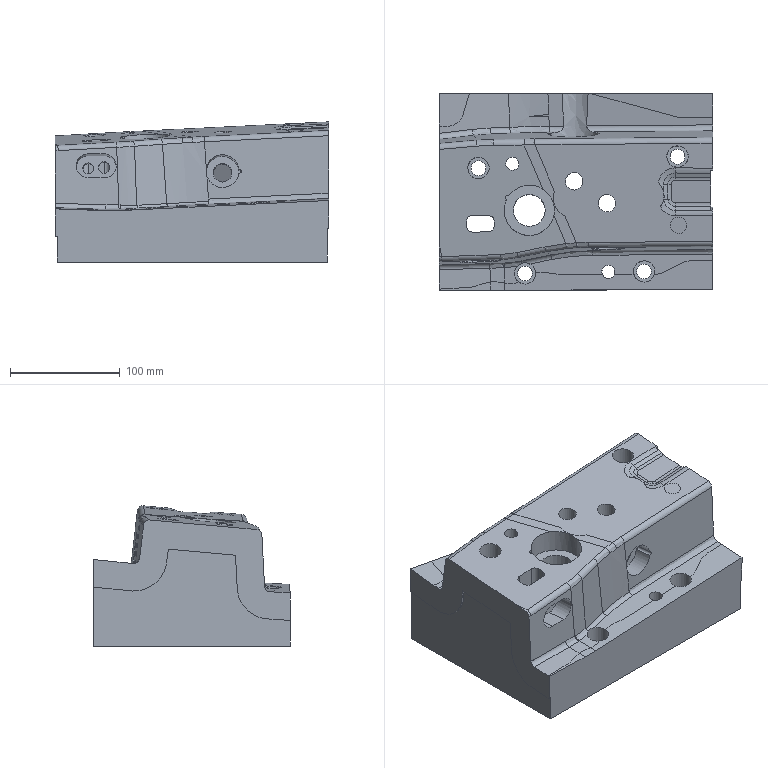Part | NX | features solid 2 | 1 solid | 145 faces | box 249.358 x 179.339 x 127.867 mm | volume 3683444 mm3 | cylinder 56 | plane 46 | spline 40 | cone 3 | commonest cylinder face diameters 10 x16 30 x5 12 x4 13.5 x4 19.5 x4 4 x3